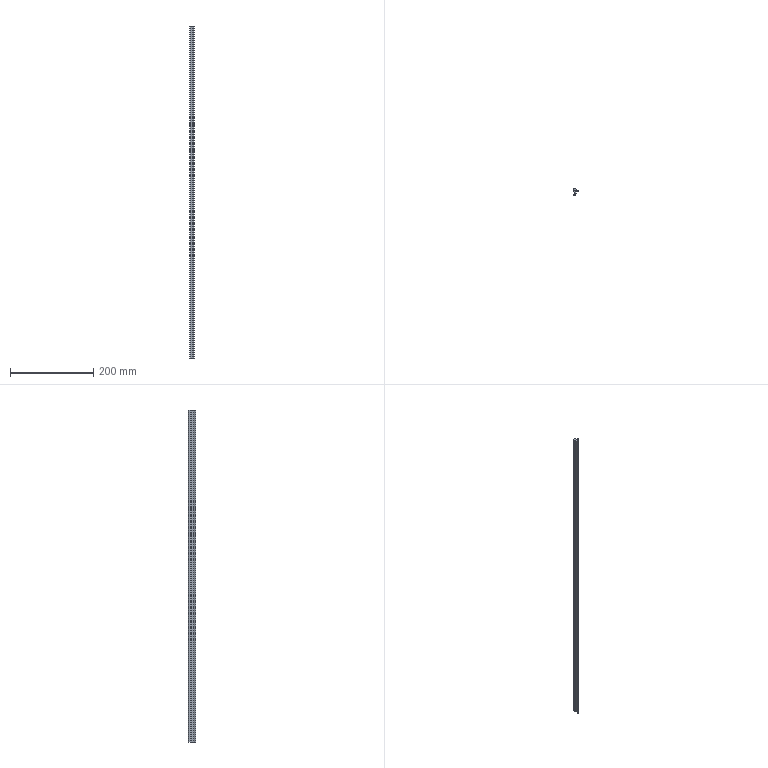Part | SolidWorks | features BaseBody 1, MoveFace 1 | 1 solid | 20 faces | box 10.8 x 17.5 x 800 mm | volume 63040 mm3 | cylinder 11 | plane 9 | commonest cylinder face diameters 1.6 x2 14 x2 0.4 x1 0.6 x1 0.8 x1 2.6 x1
STEP:
#1=CARTESIAN_POINT('',(-3.236,-11.055,700.));
#2=VERTEX_POINT('',#1);
#3=CARTESIAN_POINT('',(-4.3,-10.3,700.));
#4=VERTEX_POINT('',#3);
#5=CARTESIAN_POINT('',(-3.5,-10.3,700.));
#6=DIRECTION('',(0.,0.,-1.));
#7=DIRECTION('',(1.,0.,0.));
#8=AXIS2_PLACEMENT_3D('',#5,#6,#7);
#9=CIRCLE('',#8,0.8);
#10=EDGE_CURVE('',#2,#4,#9,.T.);
#11=ORIENTED_EDGE('',*,*,#10,.T.);
#12=CARTESIAN_POINT('',(-4.3,-10.3,-100.));
#13=VERTEX_POINT('',#12);
#14=CARTESIAN_POINT('',(-4.3,-10.3,-100.));
#15=DIRECTION('',(0.,0.,-1.));
#16=VECTOR('',#15,1000.);
#17=LINE('',#14,#16);
#18=EDGE_CURVE('',#4,#13,#17,.T.);
#19=ORIENTED_EDGE('',*,*,#18,.T.);
#20=CARTESIAN_POINT('',(-3.236,-11.055,-100.));
#21=VERTEX_POINT('',#20);
#22=CARTESIAN_POINT('',(-3.5,-10.3,-100.));
#23=DIRECTION('',(0.,0.,1.));
#24=DIRECTION('',(-1.,0.,0.));
#25=AXIS2_PLACEMENT_3D('',#22,#23,#24);
#26=CIRCLE('',#25,0.8);
#27=EDGE_CURVE('',#13,#21,#26,.T.);
#28=ORIENTED_EDGE('',*,*,#27,.T.);
#29=CARTESIAN_POINT('',(-3.236,-11.055,-100.));
#30=DIRECTION('',(0.,0.,-1.));
#31=VECTOR('',#30,1000.);
#32=LINE('',#29,#31);
#33=EDGE_CURVE('',#2,#21,#32,.T.);
#34=ORIENTED_EDGE('',*,*,#33,.F.);
#35=EDGE_LOOP('',(#11,#19,#28,#34));
#36=FACE_OUTER_BOUND('',#35,.T.);
#37=CARTESIAN_POINT('',(-3.5,-10.3,-100.));
#38=DIRECTION('',(0.,0.,-1.));
#39=DIRECTION('',(-1.,0.,0.));
#40=AXIS2_PLACEMENT_3D('',#37,#38,#39);
#41=CYLINDRICAL_SURFACE('',#40,0.8);
#42=ADVANCED_FACE('',(#36),#41,.T.);
#43=CARTESIAN_POINT('',(1.184,-6.397,-100.));
#44=VERTEX_POINT('',#43);
#45=CARTESIAN_POINT('',(-5.702,-4.29,-100.));
#46=DIRECTION('',(0.,0.,1.));
#47=DIRECTION('',(-1.,0.,0.));
#48=AXIS2_PLACEMENT_3D('',#45,#46,#47);
#49=CIRCLE('',#48,7.201);
#50=EDGE_CURVE('',#21,#44,#49,.T.);
#51=ORIENTED_EDGE('',*,*,#50,.T.);
#52=CARTESIAN_POINT('',(1.184,-6.397,700.));
#53=VERTEX_POINT('',#52);
#54=CARTESIAN_POINT('',(1.184,-6.397,-100.));
#55=DIRECTION('',(0.,0.,1.));
#56=VECTOR('',#55,1000.);
#57=LINE('',#54,#56);
#58=EDGE_CURVE('',#44,#53,#57,.T.);
#59=ORIENTED_EDGE('',*,*,#58,.T.);
#60=CARTESIAN_POINT('',(-5.702,-4.29,700.));
#61=DIRECTION('',(0.,0.,-1.));
#62=DIRECTION('',(1.,0.,0.));
#63=AXIS2_PLACEMENT_3D('',#60,#61,#62);
#64=CIRCLE('',#63,7.201);
#65=EDGE_CURVE('',#53,#2,#64,.T.);
#66=ORIENTED_EDGE('',*,*,#65,.T.);
#67=ORIENTED_EDGE('',*,*,#33,.T.);
#68=EDGE_LOOP('',(#51,#59,#66,#67));
#69=FACE_OUTER_BOUND('',#68,.T.);
#70=CARTESIAN_POINT('',(-5.702,-4.29,-100.));
#71=DIRECTION('',(0.,0.,-1.));
#72=DIRECTION('',(-1.,0.,0.));
#73=AXIS2_PLACEMENT_3D('',#70,#71,#72);
#74=CYLINDRICAL_SURFACE('',#73,7.201);
#75=ADVANCED_FACE('',(#69),#74,.T.);
#76=CARTESIAN_POINT('',(0.9,-6.,-100.));
#77=VERTEX_POINT('',#76);
#78=CARTESIAN_POINT('',(0.9,-6.3,-100.));
#79=DIRECTION('',(0.,0.,1.));
#80=DIRECTION('',(-1.,0.,0.));
#81=AXIS2_PLACEMENT_3D('',#78,#79,#80);
#82=CIRCLE('',#81,0.3);
#83=EDGE_CURVE('',#44,#77,#82,.T.);
#84=ORIENTED_EDGE('',*,*,#83,.T.);
#85=CARTESIAN_POINT('',(0.9,-6.,700.));
#86=VERTEX_POINT('',#85);
#87=CARTESIAN_POINT('',(0.9,-6.,-100.));
#88=DIRECTION('',(0.,0.,1.));
#89=VECTOR('',#88,1000.);
#90=LINE('',#87,#89);
#91=EDGE_CURVE('',#77,#86,#90,.T.);
#92=ORIENTED_EDGE('',*,*,#91,.T.);
#93=CARTESIAN_POINT('',(0.9,-6.3,700.));
#94=DIRECTION('',(0.,0.,-1.));
#95=DIRECTION('',(1.,0.,0.));
#96=AXIS2_PLACEMENT_3D('',#93,#94,#95);
#97=CIRCLE('',#96,0.3);
#98=EDGE_CURVE('',#86,#53,#97,.T.);
#99=ORIENTED_EDGE('',*,*,#98,.T.);
#100=ORIENTED_EDGE('',*,*,#58,.F.);
#101=EDGE_LOOP('',(#84,#92,#99,#100));
#102=FACE_OUTER_BOUND('',#101,.T.);
#103=CARTESIAN_POINT('',(0.9,-6.3,-100.));
#104=DIRECTION('',(0.,0.,-1.));
#105=DIRECTION('',(-1.,0.,0.));
#106=AXIS2_PLACEMENT_3D('',#103,#104,#105);
#107=CYLINDRICAL_SURFACE('',#106,0.3);
#108=ADVANCED_FACE('',(#102),#107,.T.);
#109=CARTESIAN_POINT('',(-2.5,-0.5,-100.));
#110=VERTEX_POINT('',#109);
#111=CARTESIAN_POINT('',(-2.5,-6.153,-100.));
#112=VERTEX_POINT('',#111);
#113=CARTESIAN_POINT('',(-2.5,-6.397,-100.));
#114=DIRECTION('',(0.,-1.,0.));
#115=VECTOR('',#114,1000.);
#116=LINE('',#113,#115);
#117=EDGE_CURVE('',#110,#112,#116,.T.);
#118=ORIENTED_EDGE('',*,*,#117,.F.);
#119=CARTESIAN_POINT('',(-4.2,1.695,-100.));
#120=VERTEX_POINT('',#119);
#121=CARTESIAN_POINT('',(-1.701,1.875,-100.));
#122=DIRECTION('',(0.,0.,1.));
#123=DIRECTION('',(-1.,0.,0.));
#124=AXIS2_PLACEMENT_3D('',#121,#122,#123);
#125=CIRCLE('',#124,2.506);
#126=EDGE_CURVE('',#120,#110,#125,.T.);
#127=ORIENTED_EDGE('',*,*,#126,.F.);
#128=CARTESIAN_POINT('',(-4.2,5.1,-100.));
#129=VERTEX_POINT('',#128);
#130=CARTESIAN_POINT('',(-4.2,-6.397,-100.));
#131=DIRECTION('',(0.,-1.,0.));
#132=VECTOR('',#131,1000.);
#133=LINE('',#130,#132);
#134=EDGE_CURVE('',#129,#120,#133,.T.);
#135=ORIENTED_EDGE('',*,*,#134,.F.);
#136=CARTESIAN_POINT('',(-2.892,6.4,-100.));
#137=VERTEX_POINT('',#136);
#138=CARTESIAN_POINT('',(-2.9,5.1,-100.));
#139=DIRECTION('',(0.,0.,1.));
#140=DIRECTION('',(-1.,0.,0.));
#141=AXIS2_PLACEMENT_3D('',#138,#139,#140);
#142=CIRCLE('',#141,1.3);
#143=EDGE_CURVE('',#137,#129,#142,.T.);
#144=ORIENTED_EDGE('',*,*,#143,.F.);
#145=CARTESIAN_POINT('',(0.5,5.5,-100.));
#146=VERTEX_POINT('',#145);
#147=CARTESIAN_POINT('',(-2.934,-0.5999,-100.));
#148=DIRECTION('',(0.,0.,1.));
#149=DIRECTION('',(-1.,0.,0.));
#150=AXIS2_PLACEMENT_3D('',#147,#148,#149);
#151=CIRCLE('',#150,7.);
#152=EDGE_CURVE('',#146,#137,#151,.T.);
#153=ORIENTED_EDGE('',*,*,#152,.F.);
#154=CARTESIAN_POINT('',(5.5,1.7,-100.));
#155=VERTEX_POINT('',#154);
#156=CARTESIAN_POINT('',(5.5,1.7,-100.));
#157=DIRECTION('',(-0.7962,0.6051,0.));
#158=VECTOR('',#157,1000.);
#159=LINE('',#156,#158);
#160=EDGE_CURVE('',#155,#146,#159,.T.);
#161=ORIENTED_EDGE('',*,*,#160,.F.);
#162=CARTESIAN_POINT('',(6.458,-0.2215,-100.));
#163=VERTEX_POINT('',#162);
#164=CARTESIAN_POINT('',(6.458,-0.2215,-100.));
#165=DIRECTION('',(-0.4462,0.8949,0.));
#166=VECTOR('',#165,1000.);
#167=LINE('',#164,#166);
#168=EDGE_CURVE('',#163,#155,#167,.T.);
#169=ORIENTED_EDGE('',*,*,#168,.F.);
#170=CARTESIAN_POINT('',(5.895,-0.7433,-100.));
#171=VERTEX_POINT('',#170);
#172=CARTESIAN_POINT('',(6.1,-0.4,-100.));
#173=DIRECTION('',(0.,0.,1.));
#174=DIRECTION('',(-1.,0.,0.));
#175=AXIS2_PLACEMENT_3D('',#172,#173,#174);
#176=CIRCLE('',#175,0.4);
#177=EDGE_CURVE('',#171,#163,#176,.T.);
#178=ORIENTED_EDGE('',*,*,#177,.F.);
#179=CARTESIAN_POINT('',(3.,0.,-100.));
#180=VERTEX_POINT('',#179);
#181=CARTESIAN_POINT('',(2.746,-6.995,-100.));
#182=DIRECTION('',(0.,0.,-1.));
#183=DIRECTION('',(-1.,0.,0.));
#184=AXIS2_PLACEMENT_3D('',#181,#182,#183);
#185=CIRCLE('',#184,7.);
#186=EDGE_CURVE('',#180,#171,#185,.T.);
#187=ORIENTED_EDGE('',*,*,#186,.F.);
#188=CARTESIAN_POINT('',(0.,0.,-100.));
#189=VERTEX_POINT('',#188);
#190=CARTESIAN_POINT('',(-6.814,0.,-100.));
#191=DIRECTION('',(1.,0.,0.));
#192=VECTOR('',#191,1000.);
#193=LINE('',#190,#192);
#194=EDGE_CURVE('',#189,#180,#193,.T.);
#195=ORIENTED_EDGE('',*,*,#194,.F.);
#196=CARTESIAN_POINT('',(0.,-5.8,-100.));
#197=VERTEX_POINT('',#196);
#198=CARTESIAN_POINT('',(0.,-6.397,-100.));
#199=DIRECTION('',(0.,1.,0.));
#200=VECTOR('',#199,1000.);
#201=LINE('',#198,#200);
#202=EDGE_CURVE('',#197,#189,#201,.T.);
#203=ORIENTED_EDGE('',*,*,#202,.F.);
#204=CARTESIAN_POINT('',(0.2,-6.,-100.));
#205=VERTEX_POINT('',#204);
#206=CARTESIAN_POINT('',(0.2,-5.8,-100.));
#207=DIRECTION('',(0.,0.,1.));
#208=DIRECTION('',(-1.,0.,0.));
#209=AXIS2_PLACEMENT_3D('',#206,#207,#208);
#210=CIRCLE('',#209,0.2);
#211=EDGE_CURVE('',#197,#205,#210,.T.);
#212=ORIENTED_EDGE('',*,*,#211,.T.);
#213=CARTESIAN_POINT('',(-6.814,-6.,-100.));
#214=DIRECTION('',(-1.,0.,0.));
#215=VECTOR('',#214,1000.);
#216=LINE('',#213,#215);
#217=EDGE_CURVE('',#77,#205,#216,.T.);
#218=ORIENTED_EDGE('',*,*,#217,.F.);
#219=ORIENTED_EDGE('',*,*,#83,.F.);
#220=ORIENTED_EDGE('',*,*,#50,.F.);
#221=ORIENTED_EDGE('',*,*,#27,.F.);
#222=CARTESIAN_POINT('',(-3.998,-9.674,-100.));
#223=VERTEX_POINT('',#222);
#224=CARTESIAN_POINT('',(-3.5,-10.3,-100.));
#225=DIRECTION('',(0.,0.,1.));
#226=DIRECTION('',(-1.,0.,0.));
#227=AXIS2_PLACEMENT_3D('',#224,#225,#226);
#228=CIRCLE('',#227,0.8);
#229=EDGE_CURVE('',#223,#13,#228,.T.);
#230=ORIENTED_EDGE('',*,*,#229,.F.);
#231=CARTESIAN_POINT('',(-6.814,-6.397,-100.));
#232=DIRECTION('',(0.,0.,-1.));
#233=DIRECTION('',(-1.,0.,0.));
#234=AXIS2_PLACEMENT_3D('',#231,#232,#233);
#235=CIRCLE('',#234,4.321);
#236=EDGE_CURVE('',#112,#223,#235,.T.);
#237=ORIENTED_EDGE('',*,*,#236,.F.);
#238=EDGE_LOOP('',(#118,#127,#135,#144,#153,#161,#169,#178,#187,#195,#203,#212,#218,#219,#220,#221,#230,#237));
#239=FACE_OUTER_BOUND('',#238,.T.);
#240=CARTESIAN_POINT('',(-6.814,-6.397,-100.));
#241=DIRECTION('',(0.,0.,1.));
#242=DIRECTION('',(1.,0.,0.));
#243=AXIS2_PLACEMENT_3D('',#240,#241,#242);
#244=PLANE('',#243);
#245=ADVANCED_FACE('',(#239),#244,.F.);
#246=ORIENTED_EDGE('',*,*,#18,.F.);
#247=CARTESIAN_POINT('',(-3.998,-9.674,700.));
#248=VERTEX_POINT('',#247);
#249=CARTESIAN_POINT('',(-3.5,-10.3,700.));
#250=DIRECTION('',(0.,0.,-1.));
#251=DIRECTION('',(1.,0.,0.));
#252=AXIS2_PLACEMENT_3D('',#249,#250,#251);
#253=CIRCLE('',#252,0.8);
#254=EDGE_CURVE('',#4,#248,#253,.T.);
#255=ORIENTED_EDGE('',*,*,#254,.T.);
#256=CARTESIAN_POINT('',(-3.998,-9.674,-100.));
#257=DIRECTION('',(0.,0.,-1.));
#258=VECTOR('',#257,1000.);
#259=LINE('',#256,#258);
#260=EDGE_CURVE('',#248,#223,#259,.T.);
#261=ORIENTED_EDGE('',*,*,#260,.T.);
#262=ORIENTED_EDGE('',*,*,#229,.T.);
#263=EDGE_LOOP('',(#246,#255,#261,#262));
#264=FACE_OUTER_BOUND('',#263,.T.);
#265=CARTESIAN_POINT('',(-3.5,-10.3,-100.));
#266=DIRECTION('',(0.,0.,-1.));
#267=DIRECTION('',(-1.,0.,0.));
#268=AXIS2_PLACEMENT_3D('',#265,#266,#267);
#269=CYLINDRICAL_SURFACE('',#268,0.8);
#270=ADVANCED_FACE('',(#264),#269,.T.);
#271=CARTESIAN_POINT('',(-4.2,1.695,700.));
#272=VERTEX_POINT('',#271);
#273=CARTESIAN_POINT('',(-2.5,-0.5,700.));
#274=VERTEX_POINT('',#273);
#275=CARTESIAN_POINT('',(-1.701,1.875,700.));
#276=DIRECTION('',(0.,0.,1.));
#277=DIRECTION('',(1.,0.,0.));
#278=AXIS2_PLACEMENT_3D('',#275,#276,#277);
#279=CIRCLE('',#278,2.506);
#280=EDGE_CURVE('',#272,#274,#279,.T.);
#281=ORIENTED_EDGE('',*,*,#280,.T.);
#282=CARTESIAN_POINT('',(-2.5,-6.153,700.));
#283=VERTEX_POINT('',#282);
#284=CARTESIAN_POINT('',(-2.5,-6.397,700.));
#285=DIRECTION('',(0.,-1.,0.));
#286=VECTOR('',#285,1000.);
#287=LINE('',#284,#286);
#288=EDGE_CURVE('',#274,#283,#287,.T.);
#289=ORIENTED_EDGE('',*,*,#288,.T.);
#290=CARTESIAN_POINT('',(-6.814,-6.397,700.));
#291=DIRECTION('',(0.,0.,-1.));
#292=DIRECTION('',(1.,0.,0.));
#293=AXIS2_PLACEMENT_3D('',#290,#291,#292);
#294=CIRCLE('',#293,4.321);
#295=EDGE_CURVE('',#283,#248,#294,.T.);
#296=ORIENTED_EDGE('',*,*,#295,.T.);
#297=ORIENTED_EDGE('',*,*,#254,.F.);
#298=ORIENTED_EDGE('',*,*,#10,.F.);
#299=ORIENTED_EDGE('',*,*,#65,.F.);
#300=ORIENTED_EDGE('',*,*,#98,.F.);
#301=CARTESIAN_POINT('',(0.2,-6.,700.));
#302=VERTEX_POINT('',#301);
#303=CARTESIAN_POINT('',(-6.814,-6.,700.));
#304=DIRECTION('',(-1.,0.,0.));
#305=VECTOR('',#304,1000.);
#306=LINE('',#303,#305);
#307=EDGE_CURVE('',#86,#302,#306,.T.);
#308=ORIENTED_EDGE('',*,*,#307,.T.);
#309=CARTESIAN_POINT('',(0.,-5.8,700.));
#310=VERTEX_POINT('',#309);
#311=CARTESIAN_POINT('',(0.2,-5.8,700.));
#312=DIRECTION('',(0.,0.,-1.));
#313=DIRECTION('',(1.,0.,0.));
#314=AXIS2_PLACEMENT_3D('',#311,#312,#313);
#315=CIRCLE('',#314,0.2);
#316=EDGE_CURVE('',#302,#310,#315,.T.);
#317=ORIENTED_EDGE('',*,*,#316,.T.);
#318=CARTESIAN_POINT('',(0.,0.,700.));
#319=VERTEX_POINT('',#318);
#320=CARTESIAN_POINT('',(0.,-6.397,700.));
#321=DIRECTION('',(0.,1.,0.));
#322=VECTOR('',#321,1000.);
#323=LINE('',#320,#322);
#324=EDGE_CURVE('',#310,#319,#323,.T.);
#325=ORIENTED_EDGE('',*,*,#324,.T.);
#326=CARTESIAN_POINT('',(3.,0.,700.));
#327=VERTEX_POINT('',#326);
#328=CARTESIAN_POINT('',(-6.814,0.,700.));
#329=DIRECTION('',(1.,0.,0.));
#330=VECTOR('',#329,1000.);
#331=LINE('',#328,#330);
#332=EDGE_CURVE('',#319,#327,#331,.T.);
#333=ORIENTED_EDGE('',*,*,#332,.T.);
#334=CARTESIAN_POINT('',(5.895,-0.7433,700.));
#335=VERTEX_POINT('',#334);
#336=CARTESIAN_POINT('',(2.746,-6.995,700.));
#337=DIRECTION('',(0.,0.,-1.));
#338=DIRECTION('',(1.,0.,0.));
#339=AXIS2_PLACEMENT_3D('',#336,#337,#338);
#340=CIRCLE('',#339,7.);
#341=EDGE_CURVE('',#327,#335,#340,.T.);
#342=ORIENTED_EDGE('',*,*,#341,.T.);
#343=CARTESIAN_POINT('',(6.458,-0.2215,700.));
#344=VERTEX_POINT('',#343);
#345=CARTESIAN_POINT('',(6.1,-0.4,700.));
#346=DIRECTION('',(0.,0.,-1.));
#347=DIRECTION('',(1.,0.,0.));
#348=AXIS2_PLACEMENT_3D('',#345,#346,#347);
#349=CIRCLE('',#348,0.4);
#350=EDGE_CURVE('',#344,#335,#349,.T.);
#351=ORIENTED_EDGE('',*,*,#350,.F.);
#352=CARTESIAN_POINT('',(5.5,1.7,700.));
#353=VERTEX_POINT('',#352);
#354=CARTESIAN_POINT('',(6.282,0.1323,700.));
#355=DIRECTION('',(-0.4462,0.8949,0.));
#356=VECTOR('',#355,1000.);
#357=LINE('',#354,#356);
#358=EDGE_CURVE('',#344,#353,#357,.T.);
#359=ORIENTED_EDGE('',*,*,#358,.T.);
#360=CARTESIAN_POINT('',(0.5,5.5,700.));
#361=VERTEX_POINT('',#360);
#362=CARTESIAN_POINT('',(1.595,4.668,700.));
#363=DIRECTION('',(-0.7962,0.6051,0.));
#364=VECTOR('',#363,1000.);
#365=LINE('',#362,#364);
#366=EDGE_CURVE('',#353,#361,#365,.T.);
#367=ORIENTED_EDGE('',*,*,#366,.T.);
#368=CARTESIAN_POINT('',(-2.892,6.4,700.));
#369=VERTEX_POINT('',#368);
#370=CARTESIAN_POINT('',(-2.934,-0.5999,700.));
#371=DIRECTION('',(0.,0.,1.));
#372=DIRECTION('',(1.,0.,0.));
#373=AXIS2_PLACEMENT_3D('',#370,#371,#372);
#374=CIRCLE('',#373,7.);
#375=EDGE_CURVE('',#361,#369,#374,.T.);
#376=ORIENTED_EDGE('',*,*,#375,.T.);
#377=CARTESIAN_POINT('',(-4.2,5.1,700.));
#378=VERTEX_POINT('',#377);
#379=CARTESIAN_POINT('',(-2.9,5.1,700.));
#380=DIRECTION('',(0.,0.,1.));
#381=DIRECTION('',(1.,0.,0.));
#382=AXIS2_PLACEMENT_3D('',#379,#380,#381);
#383=CIRCLE('',#382,1.3);
#384=EDGE_CURVE('',#369,#378,#383,.T.);
#385=ORIENTED_EDGE('',*,*,#384,.T.);
#386=CARTESIAN_POINT('',(-4.2,-6.397,700.));
#387=DIRECTION('',(0.,-1.,0.));
#388=VECTOR('',#387,1000.);
#389=LINE('',#386,#388);
#390=EDGE_CURVE('',#378,#272,#389,.T.);
#391=ORIENTED_EDGE('',*,*,#390,.T.);
#392=EDGE_LOOP('',(#281,#289,#296,#297,#298,#299,#300,#308,#317,#325,#333,#342,#351,#359,#367,#376,#385,#391));
#393=FACE_OUTER_BOUND('',#392,.T.);
#394=CARTESIAN_POINT('',(-6.814,-6.397,700.));
#395=DIRECTION('',(0.,0.,1.));
#396=DIRECTION('',(1.,0.,0.));
#397=AXIS2_PLACEMENT_3D('',#394,#395,#396);
#398=PLANE('',#397);
#399=ADVANCED_FACE('',(#393),#398,.T.);
#400=ORIENTED_EDGE('',*,*,#217,.T.);
#401=CARTESIAN_POINT('',(0.2,-6.,-100.));
#402=DIRECTION('',(0.,0.,1.));
#403=VECTOR('',#402,1000.);
#404=LINE('',#401,#403);
#405=EDGE_CURVE('',#205,#302,#404,.T.);
#406=ORIENTED_EDGE('',*,*,#405,.T.);
#407=ORIENTED_EDGE('',*,*,#307,.F.);
#408=ORIENTED_EDGE('',*,*,#91,.F.);
#409=EDGE_LOOP('',(#400,#406,#407,#408));
#410=FACE_OUTER_BOUND('',#409,.T.);
#411=CARTESIAN_POINT('',(0.9,-6.,-100.));
#412=DIRECTION('',(0.,1.,0.));
#413=DIRECTION('',(0.,0.,1.));
#414=AXIS2_PLACEMENT_3D('',#411,#412,#413);
#415=PLANE('',#414);
#416=ADVANCED_FACE('',(#410),#415,.T.);
#417=CARTESIAN_POINT('',(-2.5,-6.153,-100.));
#418=DIRECTION('',(0.,0.,1.));
#419=VECTOR('',#418,1000.);
#420=LINE('',#417,#419);
#421=EDGE_CURVE('',#112,#283,#420,.T.);
#422=ORIENTED_EDGE('',*,*,#421,.F.);
#423=ORIENTED_EDGE('',*,*,#236,.T.);
#424=ORIENTED_EDGE('',*,*,#260,.F.);
#425=ORIENTED_EDGE('',*,*,#295,.F.);
#426=EDGE_LOOP('',(#422,#423,#424,#425));
#427=FACE_OUTER_BOUND('',#426,.T.);
#428=CARTESIAN_POINT('',(-6.814,-6.397,-100.));
#429=DIRECTION('',(0.,0.,-1.));
#430=DIRECTION('',(-1.,0.,0.));
#431=AXIS2_PLACEMENT_3D('',#428,#429,#430);
#432=CYLINDRICAL_SURFACE('',#431,4.321);
#433=ADVANCED_FACE('',(#427),#432,.F.);
#434=ORIENTED_EDGE('',*,*,#117,.T.);
#435=ORIENTED_EDGE('',*,*,#421,.T.);
#436=ORIENTED_EDGE('',*,*,#288,.F.);
#437=CARTESIAN_POINT('',(-2.5,-0.5,-100.));
#438=DIRECTION('',(0.,0.,-1.));
#439=VECTOR('',#438,1000.);
#440=LINE('',#437,#439);
#441=EDGE_CURVE('',#274,#110,#440,.T.);
#442=ORIENTED_EDGE('',*,*,#441,.T.);
#443=EDGE_LOOP('',(#434,#435,#436,#442));
#444=FACE_OUTER_BOUND('',#443,.T.);
#445=CARTESIAN_POINT('',(-2.5,-0.5,-100.));
#446=DIRECTION('',(-1.,0.,0.));
#447=DIRECTION('',(0.,0.,1.));
#448=AXIS2_PLACEMENT_3D('',#445,#446,#447);
#449=PLANE('',#448);
#450=ADVANCED_FACE('',(#444),#449,.T.);
#451=ORIENTED_EDGE('',*,*,#126,.T.);
#452=ORIENTED_EDGE('',*,*,#441,.F.);
#453=ORIENTED_EDGE('',*,*,#280,.F.);
#454=CARTESIAN_POINT('',(-4.2,1.695,-100.));
#455=DIRECTION('',(0.,0.,-1.));
#456=VECTOR('',#455,1000.);
#457=LINE('',#454,#456);
#458=EDGE_CURVE('',#272,#120,#457,.T.);
#459=ORIENTED_EDGE('',*,*,#458,.T.);
#460=EDGE_LOOP('',(#451,#452,#453,#459));
#461=FACE_OUTER_BOUND('',#460,.T.);
#462=CARTESIAN_POINT('',(-1.701,1.875,-100.));
#463=DIRECTION('',(0.,0.,-1.));
#464=DIRECTION('',(-1.,0.,0.));
#465=AXIS2_PLACEMENT_3D('',#462,#463,#464);
#466=CYLINDRICAL_SURFACE('',#465,2.506);
#467=ADVANCED_FACE('',(#461),#466,.T.);
#468=ORIENTED_EDGE('',*,*,#134,.T.);
#469=ORIENTED_EDGE('',*,*,#458,.F.);
#470=ORIENTED_EDGE('',*,*,#390,.F.);
#471=CARTESIAN_POINT('',(-4.2,5.1,-100.));
#472=DIRECTION('',(0.,0.,-1.));
#473=VECTOR('',#472,1000.);
#474=LINE('',#471,#473);
#475=EDGE_CURVE('',#378,#129,#474,.T.);
#476=ORIENTED_EDGE('',*,*,#475,.T.);
#477=EDGE_LOOP('',(#468,#469,#470,#476));
#478=FACE_OUTER_BOUND('',#477,.T.);
#479=CARTESIAN_POINT('',(-4.2,5.1,-100.));
#480=DIRECTION('',(-1.,0.,0.));
#481=DIRECTION('',(0.,0.,1.));
#482=AXIS2_PLACEMENT_3D('',#479,#480,#481);
#483=PLANE('',#482);
#484=ADVANCED_FACE('',(#478),#483,.T.);
#485=ORIENTED_EDGE('',*,*,#143,.T.);
#486=ORIENTED_EDGE('',*,*,#475,.F.);
#487=ORIENTED_EDGE('',*,*,#384,.F.);
#488=CARTESIAN_POINT('',(-2.892,6.4,-100.));
#489=DIRECTION('',(0.,0.,-1.));
#490=VECTOR('',#489,1000.);
#491=LINE('',#488,#490);
#492=EDGE_CURVE('',#369,#137,#491,.T.);
#493=ORIENTED_EDGE('',*,*,#492,.T.);
#494=EDGE_LOOP('',(#485,#486,#487,#493));
#495=FACE_OUTER_BOUND('',#494,.T.);
#496=CARTESIAN_POINT('',(-2.9,5.1,-100.));
#497=DIRECTION('',(0.,0.,-1.));
#498=DIRECTION('',(-1.,0.,0.));
#499=AXIS2_PLACEMENT_3D('',#496,#497,#498);
#500=CYLINDRICAL_SURFACE('',#499,1.3);
#501=ADVANCED_FACE('',(#495),#500,.T.);
#502=ORIENTED_EDGE('',*,*,#152,.T.);
#503=ORIENTED_EDGE('',*,*,#492,.F.);
#504=ORIENTED_EDGE('',*,*,#375,.F.);
#505=CARTESIAN_POINT('',(0.5,5.5,-100.));
#506=DIRECTION('',(0.,0.,-1.));
#507=VECTOR('',#506,1000.);
#508=LINE('',#505,#507);
#509=EDGE_CURVE('',#361,#146,#508,.T.);
#510=ORIENTED_EDGE('',*,*,#509,.T.);
#511=EDGE_LOOP('',(#502,#503,#504,#510));
#512=FACE_OUTER_BOUND('',#511,.T.);
#513=CARTESIAN_POINT('',(-2.934,-0.5999,-100.));
#514=DIRECTION('',(0.,0.,-1.));
#515=DIRECTION('',(-1.,0.,0.));
#516=AXIS2_PLACEMENT_3D('',#513,#514,#515);
#517=CYLINDRICAL_SURFACE('',#516,7.);
#518=ADVANCED_FACE('',(#512),#517,.T.);
#519=ORIENTED_EDGE('',*,*,#160,.T.);
#520=ORIENTED_EDGE('',*,*,#509,.F.);
#521=ORIENTED_EDGE('',*,*,#366,.F.);
#522=CARTESIAN_POINT('',(5.5,1.7,-100.));
#523=DIRECTION('',(0.,0.,-1.));
#524=VECTOR('',#523,1000.);
#525=LINE('',#522,#524);
#526=EDGE_CURVE('',#353,#155,#525,.T.);
#527=ORIENTED_EDGE('',*,*,#526,.T.);
#528=EDGE_LOOP('',(#519,#520,#521,#527));
#529=FACE_OUTER_BOUND('',#528,.T.);
#530=CARTESIAN_POINT('',(5.5,1.7,-100.));
#531=DIRECTION('',(0.6051,0.7962,0.));
#532=DIRECTION('',(-0.7962,0.6051,0.));
#533=AXIS2_PLACEMENT_3D('',#530,#531,#532);
#534=PLANE('',#533);
#535=ADVANCED_FACE('',(#529),#534,.T.);
#536=ORIENTED_EDGE('',*,*,#168,.T.);
#537=ORIENTED_EDGE('',*,*,#526,.F.);
#538=ORIENTED_EDGE('',*,*,#358,.F.);
#539=CARTESIAN_POINT('',(6.458,-0.2215,-100.));
#540=DIRECTION('',(0.,0.,-1.));
#541=VECTOR('',#540,1000.);
#542=LINE('',#539,#541);
#543=EDGE_CURVE('',#344,#163,#542,.T.);
#544=ORIENTED_EDGE('',*,*,#543,.T.);
#545=EDGE_LOOP('',(#536,#537,#538,#544));
#546=FACE_OUTER_BOUND('',#545,.T.);
#547=CARTESIAN_POINT('',(6.458,-0.2215,-100.));
#548=DIRECTION('',(0.8949,0.4462,0.));
#549=DIRECTION('',(-0.4462,0.8949,0.));
#550=AXIS2_PLACEMENT_3D('',#547,#548,#549);
#551=PLANE('',#550);
#552=ADVANCED_FACE('',(#546),#551,.T.);
#553=CARTESIAN_POINT('',(3.,0.,-100.));
#554=DIRECTION('',(0.,0.,1.));
#555=VECTOR('',#554,1000.);
#556=LINE('',#553,#555);
#557=EDGE_CURVE('',#180,#327,#556,.T.);
#558=ORIENTED_EDGE('',*,*,#557,.F.);
#559=ORIENTED_EDGE('',*,*,#186,.T.);
#560=CARTESIAN_POINT('',(5.895,-0.7433,-100.));
#561=DIRECTION('',(0.,0.,-1.));
#562=VECTOR('',#561,1000.);
#563=LINE('',#560,#562);
#564=EDGE_CURVE('',#335,#171,#563,.T.);
#565=ORIENTED_EDGE('',*,*,#564,.F.);
#566=ORIENTED_EDGE('',*,*,#341,.F.);
#567=EDGE_LOOP('',(#558,#559,#565,#566));
#568=FACE_OUTER_BOUND('',#567,.T.);
#569=CARTESIAN_POINT('',(2.746,-6.995,-100.));
#570=DIRECTION('',(0.,0.,-1.));
#571=DIRECTION('',(-1.,0.,0.));
#572=AXIS2_PLACEMENT_3D('',#569,#570,#571);
#573=CYLINDRICAL_SURFACE('',#572,7.);
#574=ADVANCED_FACE('',(#568),#573,.F.);
#575=ORIENTED_EDGE('',*,*,#194,.T.);
#576=ORIENTED_EDGE('',*,*,#557,.T.);
#577=ORIENTED_EDGE('',*,*,#332,.F.);
#578=CARTESIAN_POINT('',(0.,0.,-100.));
#579=DIRECTION('',(0.,0.,-1.));
#580=VECTOR('',#579,1000.);
#581=LINE('',#578,#580);
#582=EDGE_CURVE('',#319,#189,#581,.T.);
#583=ORIENTED_EDGE('',*,*,#582,.T.);
#584=EDGE_LOOP('',(#575,#576,#577,#583));
#585=FACE_OUTER_BOUND('',#584,.T.);
#586=CARTESIAN_POINT('',(0.,0.,-100.));
#587=DIRECTION('',(0.,-1.,0.));
#588=DIRECTION('',(0.,0.,-1.));
#589=AXIS2_PLACEMENT_3D('',#586,#587,#588);
#590=PLANE('',#589);
#591=ADVANCED_FACE('',(#585),#590,.T.);
#592=ORIENTED_EDGE('',*,*,#202,.T.);
#593=ORIENTED_EDGE('',*,*,#582,.F.);
#594=ORIENTED_EDGE('',*,*,#324,.F.);
#595=CARTESIAN_POINT('',(0.,-5.8,-100.));
#596=DIRECTION('',(0.,0.,-1.));
#597=VECTOR('',#596,1000.);
#598=LINE('',#595,#597);
#599=EDGE_CURVE('',#310,#197,#598,.T.);
#600=ORIENTED_EDGE('',*,*,#599,.T.);
#601=EDGE_LOOP('',(#592,#593,#594,#600));
#602=FACE_OUTER_BOUND('',#601,.T.);
#603=CARTESIAN_POINT('',(0.,-5.8,-100.));
#604=DIRECTION('',(1.,0.,0.));
#605=DIRECTION('',(0.,0.,-1.));
#606=AXIS2_PLACEMENT_3D('',#603,#604,#605);
#607=PLANE('',#606);
#608=ADVANCED_FACE('',(#602),#607,.T.);
#609=ORIENTED_EDGE('',*,*,#405,.F.);
#610=ORIENTED_EDGE('',*,*,#211,.F.);
#611=ORIENTED_EDGE('',*,*,#599,.F.);
#612=ORIENTED_EDGE('',*,*,#316,.F.);
#613=EDGE_LOOP('',(#609,#610,#611,#612));
#614=FACE_OUTER_BOUND('',#613,.T.);
#615=CARTESIAN_POINT('',(0.2,-5.8,-100.));
#616=DIRECTION('',(0.,0.,-1.));
#617=DIRECTION('',(-1.,0.,0.));
#618=AXIS2_PLACEMENT_3D('',#615,#616,#617);
#619=CYLINDRICAL_SURFACE('',#618,0.2);
#620=ADVANCED_FACE('',(#614),#619,.F.);
#621=ORIENTED_EDGE('',*,*,#177,.T.);
#622=ORIENTED_EDGE('',*,*,#543,.F.);
#623=ORIENTED_EDGE('',*,*,#350,.T.);
#624=ORIENTED_EDGE('',*,*,#564,.T.);
#625=EDGE_LOOP('',(#621,#622,#623,#624));
#626=FACE_OUTER_BOUND('',#625,.T.);
#627=CARTESIAN_POINT('',(6.1,-0.4,-100.));
#628=DIRECTION('',(0.,0.,-1.));
#629=DIRECTION('',(-1.,0.,0.));
#630=AXIS2_PLACEMENT_3D('',#627,#628,#629);
#631=CYLINDRICAL_SURFACE('',#630,0.4);
#632=ADVANCED_FACE('',(#626),#631,.T.);
#633=CLOSED_SHELL('',(#42,#75,#108,#245,#270,#399,#416,#433,#450,#467,#484,#501,#518,#535,#552,#574,#591,#608,#620,#632));
#634=MANIFOLD_SOLID_BREP('',#633);
#635=CARTESIAN_POINT('',(0.,0.,0.));
#636=DIRECTION('',(0.,0.,1.));
#637=DIRECTION('',(1.,0.,0.));
#638=AXIS2_PLACEMENT_3D('',#635,#636,#637);
#639=(LENGTH_UNIT()NAMED_UNIT(*)SI_UNIT(.MILLI.,.METRE.));
#640=UNCERTAINTY_MEASURE_WITH_UNIT(LENGTH_MEASURE(0.00001),#639,'','');
#641=(NAMED_UNIT(*)PLANE_ANGLE_UNIT()SI_UNIT($,.RADIAN.));
#642=(NAMED_UNIT(*)SI_UNIT($,.STERADIAN.)SOLID_ANGLE_UNIT());
#643=(GEOMETRIC_REPRESENTATION_CONTEXT(3)GLOBAL_UNCERTAINTY_ASSIGNED_CONTEXT((#640))GLOBAL_UNIT_ASSIGNED_CONTEXT((#639,#641,#642))REPRESENTATION_CONTEXT('',''));
#644=ADVANCED_BREP_SHAPE_REPRESENTATION('',(#634,#638),#643);